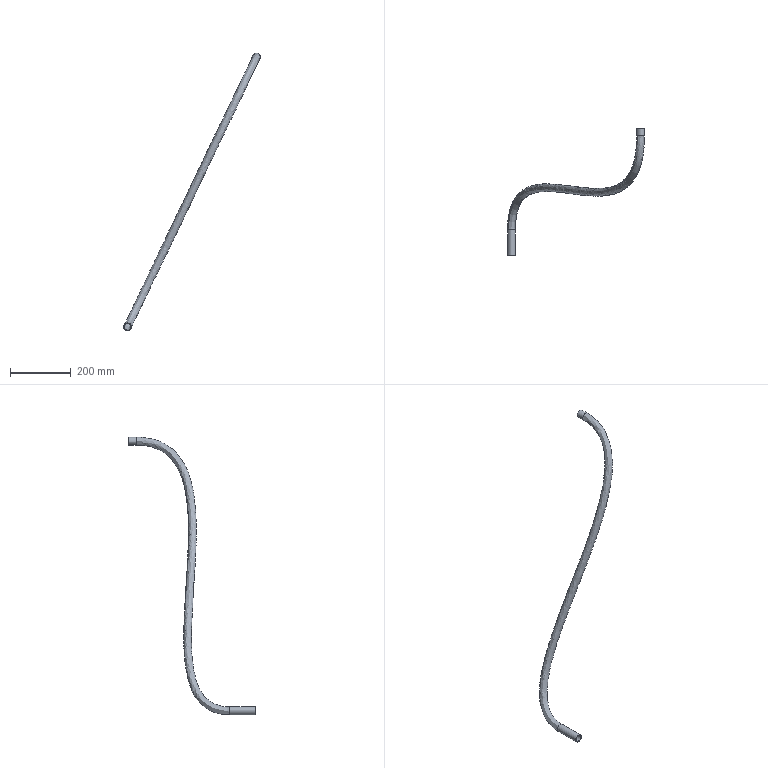Part | STEP file | Part 7^JBJ-F-0000-00 | 1 solid | 8 faces | box 451.097 x 417.992 x 914.606 mm | volume 190642 mm3 | cylinder 4 | spline 2 | plane 2 | commonest cylinder face diameters 22 x2 26 x2